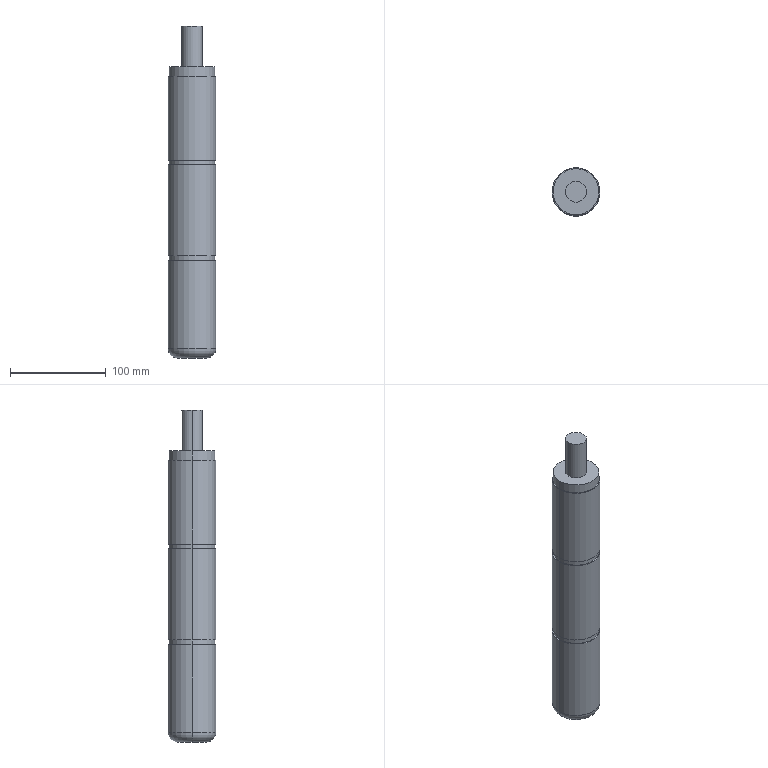Part | SolidWorks | features BaseBody 1 | 1 solid | 24 faces | box 50 x 50 x 346.5 mm | volume 606763 mm3 | cylinder 14 | plane 8 | torus 2 | commonest cylinder face diameters 48 x6 50 x6 21.9 x2
STEP:
#1=CARTESIAN_POINT('',(10.95,0.,346.5));
#2=VERTEX_POINT('',#1);
#3=CARTESIAN_POINT('',(-10.95,0.,346.5));
#4=VERTEX_POINT('',#3);
#5=CARTESIAN_POINT('',(0.,0.,346.5));
#6=DIRECTION('',(0.,0.,1.));
#7=DIRECTION('',(1.,0.,0.));
#8=AXIS2_PLACEMENT_3D('',#5,#6,#7);
#9=CIRCLE('',#8,10.95);
#10=EDGE_CURVE('',#2,#4,#9,.T.);
#11=ORIENTED_EDGE('',*,*,#10,.F.);
#12=CARTESIAN_POINT('',(10.95,0.,304.));
#13=VERTEX_POINT('',#12);
#14=CARTESIAN_POINT('',(10.95,0.,346.5));
#15=DIRECTION('',(0.,0.,-1.));
#16=VECTOR('',#15,1000.);
#17=LINE('',#14,#16);
#18=EDGE_CURVE('',#2,#13,#17,.T.);
#19=ORIENTED_EDGE('',*,*,#18,.T.);
#20=CARTESIAN_POINT('',(-10.95,0.,304.));
#21=VERTEX_POINT('',#20);
#22=CARTESIAN_POINT('',(0.,0.,304.));
#23=DIRECTION('',(0.,0.,1.));
#24=DIRECTION('',(1.,0.,0.));
#25=AXIS2_PLACEMENT_3D('',#22,#23,#24);
#26=CIRCLE('',#25,10.95);
#27=EDGE_CURVE('',#13,#21,#26,.T.);
#28=ORIENTED_EDGE('',*,*,#27,.T.);
#29=CARTESIAN_POINT('',(-10.95,0.,346.5));
#30=DIRECTION('',(0.,0.,-1.));
#31=VECTOR('',#30,1000.);
#32=LINE('',#29,#31);
#33=EDGE_CURVE('',#4,#21,#32,.T.);
#34=ORIENTED_EDGE('',*,*,#33,.F.);
#35=EDGE_LOOP('',(#11,#19,#28,#34));
#36=FACE_OUTER_BOUND('',#35,.T.);
#37=CARTESIAN_POINT('',(0.,0.,346.5));
#38=DIRECTION('',(0.,0.,-1.));
#39=DIRECTION('',(-1.,0.,0.));
#40=AXIS2_PLACEMENT_3D('',#37,#38,#39);
#41=CYLINDRICAL_SURFACE('',#40,10.95);
#42=ADVANCED_FACE('',(#36),#41,.T.);
#43=CARTESIAN_POINT('',(24.,0.,294.));
#44=VERTEX_POINT('',#43);
#45=CARTESIAN_POINT('',(-24.,0.,294.));
#46=VERTEX_POINT('',#45);
#47=CARTESIAN_POINT('',(0.,0.,294.));
#48=DIRECTION('',(0.,0.,1.));
#49=DIRECTION('',(1.,0.,0.));
#50=AXIS2_PLACEMENT_3D('',#47,#48,#49);
#51=CIRCLE('',#50,24.);
#52=EDGE_CURVE('',#44,#46,#51,.T.);
#53=ORIENTED_EDGE('',*,*,#52,.T.);
#54=CARTESIAN_POINT('',(-24.,0.,304.));
#55=VERTEX_POINT('',#54);
#56=CARTESIAN_POINT('',(-24.,0.,294.));
#57=DIRECTION('',(0.,0.,1.));
#58=VECTOR('',#57,1000.);
#59=LINE('',#56,#58);
#60=EDGE_CURVE('',#46,#55,#59,.T.);
#61=ORIENTED_EDGE('',*,*,#60,.T.);
#62=CARTESIAN_POINT('',(24.,0.,304.));
#63=VERTEX_POINT('',#62);
#64=CARTESIAN_POINT('',(0.,0.,304.));
#65=DIRECTION('',(0.,0.,1.));
#66=DIRECTION('',(1.,0.,0.));
#67=AXIS2_PLACEMENT_3D('',#64,#65,#66);
#68=CIRCLE('',#67,24.);
#69=EDGE_CURVE('',#63,#55,#68,.T.);
#70=ORIENTED_EDGE('',*,*,#69,.F.);
#71=CARTESIAN_POINT('',(24.,0.,294.));
#72=DIRECTION('',(0.,0.,1.));
#73=VECTOR('',#72,1000.);
#74=LINE('',#71,#73);
#75=EDGE_CURVE('',#44,#63,#74,.T.);
#76=ORIENTED_EDGE('',*,*,#75,.F.);
#77=EDGE_LOOP('',(#53,#61,#70,#76));
#78=FACE_OUTER_BOUND('',#77,.T.);
#79=CARTESIAN_POINT('',(0.,0.,294.));
#80=DIRECTION('',(0.,0.,1.));
#81=DIRECTION('',(1.,0.,0.));
#82=AXIS2_PLACEMENT_3D('',#79,#80,#81);
#83=CYLINDRICAL_SURFACE('',#82,24.);
#84=ADVANCED_FACE('',(#78),#83,.T.);
#85=CARTESIAN_POINT('',(-15.,0.,0.));
#86=VERTEX_POINT('',#85);
#87=CARTESIAN_POINT('',(15.,0.,0.));
#88=VERTEX_POINT('',#87);
#89=CARTESIAN_POINT('',(0.,0.,0.));
#90=DIRECTION('',(0.,0.,-1.));
#91=DIRECTION('',(1.,0.,0.));
#92=AXIS2_PLACEMENT_3D('',#89,#90,#91);
#93=CIRCLE('',#92,15.);
#94=EDGE_CURVE('',#86,#88,#93,.T.);
#95=ORIENTED_EDGE('',*,*,#94,.F.);
#96=CARTESIAN_POINT('',(-25.,0.,10.));
#97=VERTEX_POINT('',#96);
#98=CARTESIAN_POINT('',(-15.,0.,10.));
#99=DIRECTION('',(0.,1.,0.));
#100=DIRECTION('',(-1.,0.,0.));
#101=AXIS2_PLACEMENT_3D('',#98,#99,#100);
#102=CIRCLE('',#101,10.);
#103=EDGE_CURVE('',#86,#97,#102,.T.);
#104=ORIENTED_EDGE('',*,*,#103,.T.);
#105=CARTESIAN_POINT('',(25.,0.,10.));
#106=VERTEX_POINT('',#105);
#107=CARTESIAN_POINT('',(0.,0.,10.));
#108=DIRECTION('',(0.,0.,1.));
#109=DIRECTION('',(1.,0.,0.));
#110=AXIS2_PLACEMENT_3D('',#107,#108,#109);
#111=CIRCLE('',#110,25.);
#112=EDGE_CURVE('',#106,#97,#111,.T.);
#113=ORIENTED_EDGE('',*,*,#112,.F.);
#114=CARTESIAN_POINT('',(15.,0.,10.));
#115=DIRECTION('',(0.,-1.,0.));
#116=DIRECTION('',(0.,0.,-1.));
#117=AXIS2_PLACEMENT_3D('',#114,#115,#116);
#118=CIRCLE('',#117,10.);
#119=EDGE_CURVE('',#88,#106,#118,.T.);
#120=ORIENTED_EDGE('',*,*,#119,.F.);
#121=EDGE_LOOP('',(#95,#104,#113,#120));
#122=FACE_OUTER_BOUND('',#121,.T.);
#123=CARTESIAN_POINT('',(0.,0.,10.));
#124=DIRECTION('',(0.,0.,1.));
#125=DIRECTION('',(1.,0.,0.));
#126=AXIS2_PLACEMENT_3D('',#123,#124,#125);
#127=TOROIDAL_SURFACE('',#126,15.,10.);
#128=ADVANCED_FACE('',(#122),#127,.T.);
#129=CARTESIAN_POINT('',(-24.,0.,206.5));
#130=VERTEX_POINT('',#129);
#131=CARTESIAN_POINT('',(24.,0.,206.5));
#132=VERTEX_POINT('',#131);
#133=CARTESIAN_POINT('',(0.,0.,206.5));
#134=DIRECTION('',(0.,0.,-1.));
#135=DIRECTION('',(-1.,0.,0.));
#136=AXIS2_PLACEMENT_3D('',#133,#134,#135);
#137=CIRCLE('',#136,24.);
#138=EDGE_CURVE('',#130,#132,#137,.T.);
#139=ORIENTED_EDGE('',*,*,#138,.T.);
#140=CARTESIAN_POINT('',(24.,0.,201.5));
#141=VERTEX_POINT('',#140);
#142=CARTESIAN_POINT('',(24.,0.,206.5));
#143=DIRECTION('',(0.,0.,-1.));
#144=VECTOR('',#143,1000.);
#145=LINE('',#142,#144);
#146=EDGE_CURVE('',#132,#141,#145,.T.);
#147=ORIENTED_EDGE('',*,*,#146,.T.);
#148=CARTESIAN_POINT('',(-24.,0.,201.5));
#149=VERTEX_POINT('',#148);
#150=CARTESIAN_POINT('',(0.,0.,201.5));
#151=DIRECTION('',(0.,0.,-1.));
#152=DIRECTION('',(-1.,0.,0.));
#153=AXIS2_PLACEMENT_3D('',#150,#151,#152);
#154=CIRCLE('',#153,24.);
#155=EDGE_CURVE('',#149,#141,#154,.T.);
#156=ORIENTED_EDGE('',*,*,#155,.F.);
#157=CARTESIAN_POINT('',(-24.,0.,206.5));
#158=DIRECTION('',(0.,0.,-1.));
#159=VECTOR('',#158,1000.);
#160=LINE('',#157,#159);
#161=EDGE_CURVE('',#130,#149,#160,.T.);
#162=ORIENTED_EDGE('',*,*,#161,.F.);
#163=EDGE_LOOP('',(#139,#147,#156,#162));
#164=FACE_OUTER_BOUND('',#163,.T.);
#165=CARTESIAN_POINT('',(0.,0.,206.5));
#166=DIRECTION('',(0.,0.,-1.));
#167=DIRECTION('',(-1.,0.,0.));
#168=AXIS2_PLACEMENT_3D('',#165,#166,#167);
#169=CYLINDRICAL_SURFACE('',#168,24.);
#170=ADVANCED_FACE('',(#164),#169,.T.);
#171=CARTESIAN_POINT('',(-25.,0.,101.5));
#172=VERTEX_POINT('',#171);
#173=CARTESIAN_POINT('',(25.,0.,101.5));
#174=VERTEX_POINT('',#173);
#175=CARTESIAN_POINT('',(0.,0.,101.5));
#176=DIRECTION('',(0.,0.,-1.));
#177=DIRECTION('',(-1.,0.,0.));
#178=AXIS2_PLACEMENT_3D('',#175,#176,#177);
#179=CIRCLE('',#178,25.);
#180=EDGE_CURVE('',#172,#174,#179,.T.);
#181=ORIENTED_EDGE('',*,*,#180,.T.);
#182=CARTESIAN_POINT('',(25.,0.,304.));
#183=DIRECTION('',(0.,0.,-1.));
#184=VECTOR('',#183,1000.);
#185=LINE('',#182,#184);
#186=EDGE_CURVE('',#174,#106,#185,.T.);
#187=ORIENTED_EDGE('',*,*,#186,.T.);
#188=ORIENTED_EDGE('',*,*,#112,.T.);
#189=CARTESIAN_POINT('',(-25.,0.,304.));
#190=DIRECTION('',(0.,0.,-1.));
#191=VECTOR('',#190,1000.);
#192=LINE('',#189,#191);
#193=EDGE_CURVE('',#172,#97,#192,.T.);
#194=ORIENTED_EDGE('',*,*,#193,.F.);
#195=EDGE_LOOP('',(#181,#187,#188,#194));
#196=FACE_OUTER_BOUND('',#195,.T.);
#197=CARTESIAN_POINT('',(0.,0.,304.));
#198=DIRECTION('',(0.,0.,-1.));
#199=DIRECTION('',(-1.,0.,0.));
#200=AXIS2_PLACEMENT_3D('',#197,#198,#199);
#201=CYLINDRICAL_SURFACE('',#200,25.);
#202=ADVANCED_FACE('',(#196),#201,.T.);
#203=CARTESIAN_POINT('',(-24.,0.,106.5));
#204=VERTEX_POINT('',#203);
#205=CARTESIAN_POINT('',(24.,0.,106.5));
#206=VERTEX_POINT('',#205);
#207=CARTESIAN_POINT('',(0.,0.,106.5));
#208=DIRECTION('',(0.,0.,-1.));
#209=DIRECTION('',(-1.,0.,0.));
#210=AXIS2_PLACEMENT_3D('',#207,#208,#209);
#211=CIRCLE('',#210,24.);
#212=EDGE_CURVE('',#204,#206,#211,.T.);
#213=ORIENTED_EDGE('',*,*,#212,.T.);
#214=CARTESIAN_POINT('',(24.,0.,101.5));
#215=VERTEX_POINT('',#214);
#216=CARTESIAN_POINT('',(24.,0.,106.5));
#217=DIRECTION('',(0.,0.,-1.));
#218=VECTOR('',#217,1000.);
#219=LINE('',#216,#218);
#220=EDGE_CURVE('',#206,#215,#219,.T.);
#221=ORIENTED_EDGE('',*,*,#220,.T.);
#222=CARTESIAN_POINT('',(-24.,0.,101.5));
#223=VERTEX_POINT('',#222);
#224=CARTESIAN_POINT('',(0.,0.,101.5));
#225=DIRECTION('',(0.,0.,-1.));
#226=DIRECTION('',(-1.,0.,0.));
#227=AXIS2_PLACEMENT_3D('',#224,#225,#226);
#228=CIRCLE('',#227,24.);
#229=EDGE_CURVE('',#223,#215,#228,.T.);
#230=ORIENTED_EDGE('',*,*,#229,.F.);
#231=CARTESIAN_POINT('',(-24.,0.,106.5));
#232=DIRECTION('',(0.,0.,-1.));
#233=VECTOR('',#232,1000.);
#234=LINE('',#231,#233);
#235=EDGE_CURVE('',#204,#223,#234,.T.);
#236=ORIENTED_EDGE('',*,*,#235,.F.);
#237=EDGE_LOOP('',(#213,#221,#230,#236));
#238=FACE_OUTER_BOUND('',#237,.T.);
#239=CARTESIAN_POINT('',(0.,0.,106.5));
#240=DIRECTION('',(0.,0.,-1.));
#241=DIRECTION('',(-1.,0.,0.));
#242=AXIS2_PLACEMENT_3D('',#239,#240,#241);
#243=CYLINDRICAL_SURFACE('',#242,24.);
#244=ADVANCED_FACE('',(#238),#243,.T.);
#245=CARTESIAN_POINT('',(-25.,0.,201.5));
#246=VERTEX_POINT('',#245);
#247=CARTESIAN_POINT('',(25.,0.,201.5));
#248=VERTEX_POINT('',#247);
#249=CARTESIAN_POINT('',(0.,0.,201.5));
#250=DIRECTION('',(0.,0.,-1.));
#251=DIRECTION('',(-1.,0.,0.));
#252=AXIS2_PLACEMENT_3D('',#249,#250,#251);
#253=CIRCLE('',#252,25.);
#254=EDGE_CURVE('',#246,#248,#253,.T.);
#255=ORIENTED_EDGE('',*,*,#254,.T.);
#256=CARTESIAN_POINT('',(25.,0.,106.5));
#257=VERTEX_POINT('',#256);
#258=CARTESIAN_POINT('',(25.,0.,304.));
#259=DIRECTION('',(0.,0.,-1.));
#260=VECTOR('',#259,1000.);
#261=LINE('',#258,#260);
#262=EDGE_CURVE('',#248,#257,#261,.T.);
#263=ORIENTED_EDGE('',*,*,#262,.T.);
#264=CARTESIAN_POINT('',(-25.,0.,106.5));
#265=VERTEX_POINT('',#264);
#266=CARTESIAN_POINT('',(0.,0.,106.5));
#267=DIRECTION('',(0.,0.,-1.));
#268=DIRECTION('',(-1.,0.,0.));
#269=AXIS2_PLACEMENT_3D('',#266,#267,#268);
#270=CIRCLE('',#269,25.);
#271=EDGE_CURVE('',#265,#257,#270,.T.);
#272=ORIENTED_EDGE('',*,*,#271,.F.);
#273=CARTESIAN_POINT('',(-25.,0.,304.));
#274=DIRECTION('',(0.,0.,-1.));
#275=VECTOR('',#274,1000.);
#276=LINE('',#273,#275);
#277=EDGE_CURVE('',#246,#265,#276,.T.);
#278=ORIENTED_EDGE('',*,*,#277,.F.);
#279=EDGE_LOOP('',(#255,#263,#272,#278));
#280=FACE_OUTER_BOUND('',#279,.T.);
#281=CARTESIAN_POINT('',(0.,0.,304.));
#282=DIRECTION('',(0.,0.,-1.));
#283=DIRECTION('',(-1.,0.,0.));
#284=AXIS2_PLACEMENT_3D('',#281,#282,#283);
#285=CYLINDRICAL_SURFACE('',#284,25.);
#286=ADVANCED_FACE('',(#280),#285,.T.);
#287=CARTESIAN_POINT('',(25.,0.,294.));
#288=VERTEX_POINT('',#287);
#289=CARTESIAN_POINT('',(-25.,0.,294.));
#290=VERTEX_POINT('',#289);
#291=CARTESIAN_POINT('',(0.,0.,294.));
#292=DIRECTION('',(0.,0.,1.));
#293=DIRECTION('',(1.,0.,0.));
#294=AXIS2_PLACEMENT_3D('',#291,#292,#293);
#295=CIRCLE('',#294,25.);
#296=EDGE_CURVE('',#288,#290,#295,.T.);
#297=ORIENTED_EDGE('',*,*,#296,.F.);
#298=CARTESIAN_POINT('',(25.,0.,206.5));
#299=VERTEX_POINT('',#298);
#300=CARTESIAN_POINT('',(25.,0.,304.));
#301=DIRECTION('',(0.,0.,-1.));
#302=VECTOR('',#301,1000.);
#303=LINE('',#300,#302);
#304=EDGE_CURVE('',#288,#299,#303,.T.);
#305=ORIENTED_EDGE('',*,*,#304,.T.);
#306=CARTESIAN_POINT('',(-25.,0.,206.5));
#307=VERTEX_POINT('',#306);
#308=CARTESIAN_POINT('',(0.,0.,206.5));
#309=DIRECTION('',(0.,0.,-1.));
#310=DIRECTION('',(-1.,0.,0.));
#311=AXIS2_PLACEMENT_3D('',#308,#309,#310);
#312=CIRCLE('',#311,25.);
#313=EDGE_CURVE('',#307,#299,#312,.T.);
#314=ORIENTED_EDGE('',*,*,#313,.F.);
#315=CARTESIAN_POINT('',(-25.,0.,304.));
#316=DIRECTION('',(0.,0.,-1.));
#317=VECTOR('',#316,1000.);
#318=LINE('',#315,#317);
#319=EDGE_CURVE('',#290,#307,#318,.T.);
#320=ORIENTED_EDGE('',*,*,#319,.F.);
#321=EDGE_LOOP('',(#297,#305,#314,#320));
#322=FACE_OUTER_BOUND('',#321,.T.);
#323=CARTESIAN_POINT('',(0.,0.,304.));
#324=DIRECTION('',(0.,0.,-1.));
#325=DIRECTION('',(-1.,0.,0.));
#326=AXIS2_PLACEMENT_3D('',#323,#324,#325);
#327=CYLINDRICAL_SURFACE('',#326,25.);
#328=ADVANCED_FACE('',(#322),#327,.T.);
#329=CARTESIAN_POINT('',(0.,0.,304.));
#330=DIRECTION('',(0.,0.,1.));
#331=DIRECTION('',(1.,0.,0.));
#332=AXIS2_PLACEMENT_3D('',#329,#330,#331);
#333=CIRCLE('',#332,10.95);
#334=EDGE_CURVE('',#21,#13,#333,.T.);
#335=ORIENTED_EDGE('',*,*,#334,.F.);
#336=ORIENTED_EDGE('',*,*,#27,.F.);
#337=EDGE_LOOP('',(#335,#336));
#338=FACE_BOUND('',#337,.T.);
#339=ORIENTED_EDGE('',*,*,#69,.T.);
#340=CARTESIAN_POINT('',(0.,0.,304.));
#341=DIRECTION('',(0.,0.,1.));
#342=DIRECTION('',(1.,0.,0.));
#343=AXIS2_PLACEMENT_3D('',#340,#341,#342);
#344=CIRCLE('',#343,24.);
#345=EDGE_CURVE('',#55,#63,#344,.T.);
#346=ORIENTED_EDGE('',*,*,#345,.T.);
#347=EDGE_LOOP('',(#339,#346));
#348=FACE_OUTER_BOUND('',#347,.T.);
#349=CARTESIAN_POINT('',(0.,0.,304.));
#350=DIRECTION('',(0.,0.,1.));
#351=DIRECTION('',(1.,0.,0.));
#352=AXIS2_PLACEMENT_3D('',#349,#350,#351);
#353=PLANE('',#352);
#354=ADVANCED_FACE('',(#338,#348),#353,.T.);
#355=CARTESIAN_POINT('',(0.,0.,346.5));
#356=DIRECTION('',(0.,0.,1.));
#357=DIRECTION('',(1.,0.,0.));
#358=AXIS2_PLACEMENT_3D('',#355,#356,#357);
#359=CIRCLE('',#358,10.95);
#360=EDGE_CURVE('',#4,#2,#359,.T.);
#361=ORIENTED_EDGE('',*,*,#360,.T.);
#362=ORIENTED_EDGE('',*,*,#10,.T.);
#363=EDGE_LOOP('',(#361,#362));
#364=FACE_OUTER_BOUND('',#363,.T.);
#365=CARTESIAN_POINT('',(0.,0.,346.5));
#366=DIRECTION('',(0.,0.,1.));
#367=DIRECTION('',(1.,0.,0.));
#368=AXIS2_PLACEMENT_3D('',#365,#366,#367);
#369=PLANE('',#368);
#370=ADVANCED_FACE('',(#364),#369,.T.);
#371=ORIENTED_EDGE('',*,*,#52,.F.);
#372=CARTESIAN_POINT('',(0.,0.,294.));
#373=DIRECTION('',(0.,0.,1.));
#374=DIRECTION('',(1.,0.,0.));
#375=AXIS2_PLACEMENT_3D('',#372,#373,#374);
#376=CIRCLE('',#375,24.);
#377=EDGE_CURVE('',#46,#44,#376,.T.);
#378=ORIENTED_EDGE('',*,*,#377,.F.);
#379=EDGE_LOOP('',(#371,#378));
#380=FACE_BOUND('',#379,.T.);
#381=CARTESIAN_POINT('',(0.,0.,294.));
#382=DIRECTION('',(0.,0.,1.));
#383=DIRECTION('',(1.,0.,0.));
#384=AXIS2_PLACEMENT_3D('',#381,#382,#383);
#385=CIRCLE('',#384,25.);
#386=EDGE_CURVE('',#290,#288,#385,.T.);
#387=ORIENTED_EDGE('',*,*,#386,.T.);
#388=ORIENTED_EDGE('',*,*,#296,.T.);
#389=EDGE_LOOP('',(#387,#388));
#390=FACE_OUTER_BOUND('',#389,.T.);
#391=CARTESIAN_POINT('',(-1.179,0.,294.));
#392=DIRECTION('',(0.,0.,1.));
#393=DIRECTION('',(1.,0.,0.));
#394=AXIS2_PLACEMENT_3D('',#391,#392,#393);
#395=PLANE('',#394);
#396=ADVANCED_FACE('',(#380,#390),#395,.T.);
#397=ORIENTED_EDGE('',*,*,#155,.T.);
#398=CARTESIAN_POINT('',(0.,0.,201.5));
#399=DIRECTION('',(0.,0.,-1.));
#400=DIRECTION('',(-1.,0.,0.));
#401=AXIS2_PLACEMENT_3D('',#398,#399,#400);
#402=CIRCLE('',#401,24.);
#403=EDGE_CURVE('',#141,#149,#402,.T.);
#404=ORIENTED_EDGE('',*,*,#403,.T.);
#405=EDGE_LOOP('',(#397,#404));
#406=FACE_BOUND('',#405,.T.);
#407=ORIENTED_EDGE('',*,*,#254,.F.);
#408=CARTESIAN_POINT('',(0.,0.,201.5));
#409=DIRECTION('',(0.,0.,-1.));
#410=DIRECTION('',(-1.,0.,0.));
#411=AXIS2_PLACEMENT_3D('',#408,#409,#410);
#412=CIRCLE('',#411,25.);
#413=EDGE_CURVE('',#248,#246,#412,.T.);
#414=ORIENTED_EDGE('',*,*,#413,.F.);
#415=EDGE_LOOP('',(#407,#414));
#416=FACE_OUTER_BOUND('',#415,.T.);
#417=CARTESIAN_POINT('',(0.,0.,201.5));
#418=DIRECTION('',(0.,0.,-1.));
#419=DIRECTION('',(0.,-1.,0.));
#420=AXIS2_PLACEMENT_3D('',#417,#418,#419);
#421=PLANE('',#420);
#422=ADVANCED_FACE('',(#406,#416),#421,.F.);
#423=ORIENTED_EDGE('',*,*,#138,.F.);
#424=CARTESIAN_POINT('',(0.,0.,206.5));
#425=DIRECTION('',(0.,0.,-1.));
#426=DIRECTION('',(-1.,0.,0.));
#427=AXIS2_PLACEMENT_3D('',#424,#425,#426);
#428=CIRCLE('',#427,24.);
#429=EDGE_CURVE('',#132,#130,#428,.T.);
#430=ORIENTED_EDGE('',*,*,#429,.F.);
#431=EDGE_LOOP('',(#423,#430));
#432=FACE_BOUND('',#431,.T.);
#433=ORIENTED_EDGE('',*,*,#313,.T.);
#434=CARTESIAN_POINT('',(0.,0.,206.5));
#435=DIRECTION('',(0.,0.,-1.));
#436=DIRECTION('',(-1.,0.,0.));
#437=AXIS2_PLACEMENT_3D('',#434,#435,#436);
#438=CIRCLE('',#437,25.);
#439=EDGE_CURVE('',#299,#307,#438,.T.);
#440=ORIENTED_EDGE('',*,*,#439,.T.);
#441=EDGE_LOOP('',(#433,#440));
#442=FACE_OUTER_BOUND('',#441,.T.);
#443=CARTESIAN_POINT('',(0.,0.,206.5));
#444=DIRECTION('',(0.,0.,-1.));
#445=DIRECTION('',(0.,-1.,0.));
#446=AXIS2_PLACEMENT_3D('',#443,#444,#445);
#447=PLANE('',#446);
#448=ADVANCED_FACE('',(#432,#442),#447,.T.);
#449=CARTESIAN_POINT('',(0.,0.,0.));
#450=DIRECTION('',(0.,0.,-1.));
#451=DIRECTION('',(1.,0.,0.));
#452=AXIS2_PLACEMENT_3D('',#449,#450,#451);
#453=CIRCLE('',#452,15.);
#454=EDGE_CURVE('',#88,#86,#453,.T.);
#455=ORIENTED_EDGE('',*,*,#454,.T.);
#456=ORIENTED_EDGE('',*,*,#94,.T.);
#457=EDGE_LOOP('',(#455,#456));
#458=FACE_OUTER_BOUND('',#457,.T.);
#459=CARTESIAN_POINT('',(0.,0.,0.));
#460=DIRECTION('',(0.,0.,1.));
#461=DIRECTION('',(1.,0.,0.));
#462=AXIS2_PLACEMENT_3D('',#459,#460,#461);
#463=PLANE('',#462);
#464=ADVANCED_FACE('',(#458),#463,.F.);
#465=ORIENTED_EDGE('',*,*,#229,.T.);
#466=CARTESIAN_POINT('',(0.,0.,101.5));
#467=DIRECTION('',(0.,0.,-1.));
#468=DIRECTION('',(-1.,0.,0.));
#469=AXIS2_PLACEMENT_3D('',#466,#467,#468);
#470=CIRCLE('',#469,24.);
#471=EDGE_CURVE('',#215,#223,#470,.T.);
#472=ORIENTED_EDGE('',*,*,#471,.T.);
#473=EDGE_LOOP('',(#465,#472));
#474=FACE_BOUND('',#473,.T.);
#475=ORIENTED_EDGE('',*,*,#180,.F.);
#476=CARTESIAN_POINT('',(0.,0.,101.5));
#477=DIRECTION('',(0.,0.,-1.));
#478=DIRECTION('',(-1.,0.,0.));
#479=AXIS2_PLACEMENT_3D('',#476,#477,#478);
#480=CIRCLE('',#479,25.);
#481=EDGE_CURVE('',#174,#172,#480,.T.);
#482=ORIENTED_EDGE('',*,*,#481,.F.);
#483=EDGE_LOOP('',(#475,#482));
#484=FACE_OUTER_BOUND('',#483,.T.);
#485=CARTESIAN_POINT('',(0.,0.,101.5));
#486=DIRECTION('',(0.,0.,-1.));
#487=DIRECTION('',(0.,-1.,0.));
#488=AXIS2_PLACEMENT_3D('',#485,#486,#487);
#489=PLANE('',#488);
#490=ADVANCED_FACE('',(#474,#484),#489,.F.);
#491=ORIENTED_EDGE('',*,*,#212,.F.);
#492=CARTESIAN_POINT('',(0.,0.,106.5));
#493=DIRECTION('',(0.,0.,-1.));
#494=DIRECTION('',(-1.,0.,0.));
#495=AXIS2_PLACEMENT_3D('',#492,#493,#494);
#496=CIRCLE('',#495,24.);
#497=EDGE_CURVE('',#206,#204,#496,.T.);
#498=ORIENTED_EDGE('',*,*,#497,.F.);
#499=EDGE_LOOP('',(#491,#498));
#500=FACE_BOUND('',#499,.T.);
#501=ORIENTED_EDGE('',*,*,#271,.T.);
#502=CARTESIAN_POINT('',(0.,0.,106.5));
#503=DIRECTION('',(0.,0.,-1.));
#504=DIRECTION('',(-1.,0.,0.));
#505=AXIS2_PLACEMENT_3D('',#502,#503,#504);
#506=CIRCLE('',#505,25.);
#507=EDGE_CURVE('',#257,#265,#506,.T.);
#508=ORIENTED_EDGE('',*,*,#507,.T.);
#509=EDGE_LOOP('',(#501,#508));
#510=FACE_OUTER_BOUND('',#509,.T.);
#511=CARTESIAN_POINT('',(0.,0.,106.5));
#512=DIRECTION('',(0.,0.,-1.));
#513=DIRECTION('',(0.,-1.,0.));
#514=AXIS2_PLACEMENT_3D('',#511,#512,#513);
#515=PLANE('',#514);
#516=ADVANCED_FACE('',(#500,#510),#515,.T.);
#517=ORIENTED_EDGE('',*,*,#304,.F.);
#518=ORIENTED_EDGE('',*,*,#386,.F.);
#519=ORIENTED_EDGE('',*,*,#319,.T.);
#520=ORIENTED_EDGE('',*,*,#439,.F.);
#521=EDGE_LOOP('',(#517,#518,#519,#520));
#522=FACE_OUTER_BOUND('',#521,.T.);
#523=CARTESIAN_POINT('',(0.,0.,304.));
#524=DIRECTION('',(0.,0.,-1.));
#525=DIRECTION('',(-1.,0.,0.));
#526=AXIS2_PLACEMENT_3D('',#523,#524,#525);
#527=CYLINDRICAL_SURFACE('',#526,25.);
#528=ADVANCED_FACE('',(#522),#527,.T.);
#529=ORIENTED_EDGE('',*,*,#262,.F.);
#530=ORIENTED_EDGE('',*,*,#413,.T.);
#531=ORIENTED_EDGE('',*,*,#277,.T.);
#532=ORIENTED_EDGE('',*,*,#507,.F.);
#533=EDGE_LOOP('',(#529,#530,#531,#532));
#534=FACE_OUTER_BOUND('',#533,.T.);
#535=CARTESIAN_POINT('',(0.,0.,304.));
#536=DIRECTION('',(0.,0.,-1.));
#537=DIRECTION('',(-1.,0.,0.));
#538=AXIS2_PLACEMENT_3D('',#535,#536,#537);
#539=CYLINDRICAL_SURFACE('',#538,25.);
#540=ADVANCED_FACE('',(#534),#539,.T.);
#541=ORIENTED_EDGE('',*,*,#220,.F.);
#542=ORIENTED_EDGE('',*,*,#497,.T.);
#543=ORIENTED_EDGE('',*,*,#235,.T.);
#544=ORIENTED_EDGE('',*,*,#471,.F.);
#545=EDGE_LOOP('',(#541,#542,#543,#544));
#546=FACE_OUTER_BOUND('',#545,.T.);
#547=CARTESIAN_POINT('',(0.,0.,106.5));
#548=DIRECTION('',(0.,0.,-1.));
#549=DIRECTION('',(-1.,0.,0.));
#550=AXIS2_PLACEMENT_3D('',#547,#548,#549);
#551=CYLINDRICAL_SURFACE('',#550,24.);
#552=ADVANCED_FACE('',(#546),#551,.T.);
#553=ORIENTED_EDGE('',*,*,#186,.F.);
#554=ORIENTED_EDGE('',*,*,#481,.T.);
#555=ORIENTED_EDGE('',*,*,#193,.T.);
#556=CARTESIAN_POINT('',(0.,0.,10.));
#557=DIRECTION('',(0.,0.,1.));
#558=DIRECTION('',(1.,0.,0.));
#559=AXIS2_PLACEMENT_3D('',#556,#557,#558);
#560=CIRCLE('',#559,25.);
#561=EDGE_CURVE('',#97,#106,#560,.T.);
#562=ORIENTED_EDGE('',*,*,#561,.T.);
#563=EDGE_LOOP('',(#553,#554,#555,#562));
#564=FACE_OUTER_BOUND('',#563,.T.);
#565=CARTESIAN_POINT('',(0.,0.,304.));
#566=DIRECTION('',(0.,0.,-1.));
#567=DIRECTION('',(-1.,0.,0.));
#568=AXIS2_PLACEMENT_3D('',#565,#566,#567);
#569=CYLINDRICAL_SURFACE('',#568,25.);
#570=ADVANCED_FACE('',(#564),#569,.T.);
#571=ORIENTED_EDGE('',*,*,#146,.F.);
#572=ORIENTED_EDGE('',*,*,#429,.T.);
#573=ORIENTED_EDGE('',*,*,#161,.T.);
#574=ORIENTED_EDGE('',*,*,#403,.F.);
#575=EDGE_LOOP('',(#571,#572,#573,#574));
#576=FACE_OUTER_BOUND('',#575,.T.);
#577=CARTESIAN_POINT('',(0.,0.,206.5));
#578=DIRECTION('',(0.,0.,-1.));
#579=DIRECTION('',(-1.,0.,0.));
#580=AXIS2_PLACEMENT_3D('',#577,#578,#579);
#581=CYLINDRICAL_SURFACE('',#580,24.);
#582=ADVANCED_FACE('',(#576),#581,.T.);
#583=ORIENTED_EDGE('',*,*,#103,.F.);
#584=ORIENTED_EDGE('',*,*,#454,.F.);
#585=ORIENTED_EDGE('',*,*,#119,.T.);
#586=ORIENTED_EDGE('',*,*,#561,.F.);
#587=EDGE_LOOP('',(#583,#584,#585,#586));
#588=FACE_OUTER_BOUND('',#587,.T.);
#589=CARTESIAN_POINT('',(0.,0.,10.));
#590=DIRECTION('',(0.,0.,1.));
#591=DIRECTION('',(1.,0.,0.));
#592=AXIS2_PLACEMENT_3D('',#589,#590,#591);
#593=TOROIDAL_SURFACE('',#592,15.,10.);
#594=ADVANCED_FACE('',(#588),#593,.T.);
#595=ORIENTED_EDGE('',*,*,#60,.F.);
#596=ORIENTED_EDGE('',*,*,#377,.T.);
#597=ORIENTED_EDGE('',*,*,#75,.T.);
#598=ORIENTED_EDGE('',*,*,#345,.F.);
#599=EDGE_LOOP('',(#595,#596,#597,#598));
#600=FACE_OUTER_BOUND('',#599,.T.);
#601=CARTESIAN_POINT('',(0.,0.,294.));
#602=DIRECTION('',(0.,0.,1.));
#603=DIRECTION('',(1.,0.,0.));
#604=AXIS2_PLACEMENT_3D('',#601,#602,#603);
#605=CYLINDRICAL_SURFACE('',#604,24.);
#606=ADVANCED_FACE('',(#600),#605,.T.);
#607=ORIENTED_EDGE('',*,*,#18,.F.);
#608=ORIENTED_EDGE('',*,*,#360,.F.);
#609=ORIENTED_EDGE('',*,*,#33,.T.);
#610=ORIENTED_EDGE('',*,*,#334,.T.);
#611=EDGE_LOOP('',(#607,#608,#609,#610));
#612=FACE_OUTER_BOUND('',#611,.T.);
#613=CARTESIAN_POINT('',(0.,0.,346.5));
#614=DIRECTION('',(0.,0.,-1.));
#615=DIRECTION('',(-1.,0.,0.));
#616=AXIS2_PLACEMENT_3D('',#613,#614,#615);
#617=CYLINDRICAL_SURFACE('',#616,10.95);
#618=ADVANCED_FACE('',(#612),#617,.T.);
#619=CLOSED_SHELL('',(#42,#84,#128,#170,#202,#244,#286,#328,#354,#370,#396,#422,#448,#464,#490,#516,#528,#540,#552,#570,#582,#594,#606,#618));
#620=MANIFOLD_SOLID_BREP('',#619);
#621=CARTESIAN_POINT('',(0.,0.,0.));
#622=DIRECTION('',(0.,0.,1.));
#623=DIRECTION('',(1.,0.,0.));
#624=AXIS2_PLACEMENT_3D('',#621,#622,#623);
#625=(LENGTH_UNIT()NAMED_UNIT(*)SI_UNIT(.MILLI.,.METRE.));
#626=UNCERTAINTY_MEASURE_WITH_UNIT(LENGTH_MEASURE(0.00001),#625,'','');
#627=(NAMED_UNIT(*)PLANE_ANGLE_UNIT()SI_UNIT($,.RADIAN.));
#628=(NAMED_UNIT(*)SI_UNIT($,.STERADIAN.)SOLID_ANGLE_UNIT());
#629=(GEOMETRIC_REPRESENTATION_CONTEXT(3)GLOBAL_UNCERTAINTY_ASSIGNED_CONTEXT((#626))GLOBAL_UNIT_ASSIGNED_CONTEXT((#625,#627,#628))REPRESENTATION_CONTEXT('',''));
#630=ADVANCED_BREP_SHAPE_REPRESENTATION('',(#620,#624),#629);